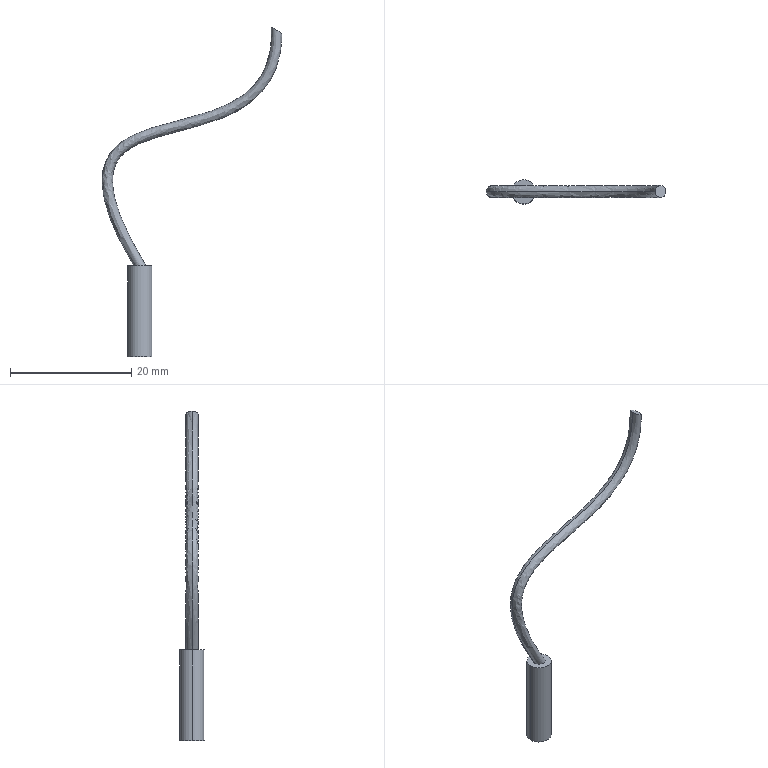Part | STEP file | Rotor detection photoelectric sensor | 1 solid | 7 faces | box 29.674 x 4 x 54.352 mm | volume 340.68 mm3 | plane 3 | spline 2 | cylinder 2 | commonest cylinder face diameters 4 x2
STEP:
#1=CARTESIAN_POINT('',(0.,0.,0.));
#2=DIRECTION('',(0.,0.,1.));
#3=DIRECTION('',(1.,0.,0.));
#4=AXIS2_PLACEMENT_3D('',#1,#2,#3);
#5=CARTESIAN_POINT('',(1.,0.,15.));
#6=VERTEX_POINT('',#5);
#7=CARTESIAN_POINT('',(-1.,0.,15.));
#8=VERTEX_POINT('',#7);
#9=CARTESIAN_POINT('',(1.,0.,15.));
#10=CARTESIAN_POINT('',(1.,2.,15.));
#11=CARTESIAN_POINT('',(-1.,2.,15.));
#12=CARTESIAN_POINT('',(-1.,0.,15.));
#13=(BOUNDED_CURVE()B_SPLINE_CURVE(3,(#9,#10,#11,#12),.UNSPECIFIED.,.F.,.F.)B_SPLINE_CURVE_WITH_KNOTS((4,4),(0.003113,0.006226),.PIECEWISE_BEZIER_KNOTS.)CURVE()GEOMETRIC_REPRESENTATION_ITEM()RATIONAL_B_SPLINE_CURVE((1.,0.3333,0.3333,1.))REPRESENTATION_ITEM(''));
#14=CARTESIAN_POINT('',(1.,0.,15.));
#15=CARTESIAN_POINT('',(0.06152,0.,16.548));
#16=CARTESIAN_POINT('',(-1.541,0.,19.409));
#17=CARTESIAN_POINT('',(-3.194,0.,23.021));
#18=CARTESIAN_POINT('',(-4.04,0.,25.6));
#19=CARTESIAN_POINT('',(-4.414,0.,27.44));
#20=CARTESIAN_POINT('',(-4.535,0.,28.749));
#21=CARTESIAN_POINT('',(-4.495,0.,29.892));
#22=CARTESIAN_POINT('',(-4.265,0.,31.131));
#23=CARTESIAN_POINT('',(-3.713,0.,32.389));
#24=CARTESIAN_POINT('',(-2.639,0.,33.627));
#25=CARTESIAN_POINT('',(-1.142,0.,34.662));
#26=CARTESIAN_POINT('',(2.557,0.,36.372));
#27=CARTESIAN_POINT('',(8.403,0.,37.548));
#28=CARTESIAN_POINT('',(14.934,0.,39.731));
#29=CARTESIAN_POINT('',(18.432,0.,41.83));
#30=CARTESIAN_POINT('',(20.585,0.,44.09));
#31=CARTESIAN_POINT('',(21.786,0.,45.892));
#32=CARTESIAN_POINT('',(22.702,0.,48.014));
#33=CARTESIAN_POINT('',(23.29,0.,50.472));
#34=CARTESIAN_POINT('',(23.436,0.,52.345));
#35=CARTESIAN_POINT('',(23.448,0.,53.346));
#36=CARTESIAN_POINT('',(1.,2.,15.));
#37=CARTESIAN_POINT('',(0.06152,2.,16.548));
#38=CARTESIAN_POINT('',(-1.541,2.,19.409));
#39=CARTESIAN_POINT('',(-3.194,2.,23.021));
#40=CARTESIAN_POINT('',(-4.04,2.,25.6));
#41=CARTESIAN_POINT('',(-4.414,2.,27.44));
#42=CARTESIAN_POINT('',(-4.535,2.,28.749));
#43=CARTESIAN_POINT('',(-4.495,2.,29.892));
#44=CARTESIAN_POINT('',(-4.265,2.,31.131));
#45=CARTESIAN_POINT('',(-3.713,2.,32.389));
#46=CARTESIAN_POINT('',(-2.639,2.,33.627));
#47=CARTESIAN_POINT('',(-1.142,2.,34.662));
#48=CARTESIAN_POINT('',(2.557,2.,36.372));
#49=CARTESIAN_POINT('',(8.403,2.,37.548));
#50=CARTESIAN_POINT('',(14.934,2.,39.731));
#51=CARTESIAN_POINT('',(18.432,2.,41.83));
#52=CARTESIAN_POINT('',(20.585,2.,44.09));
#53=CARTESIAN_POINT('',(21.786,2.,45.892));
#54=CARTESIAN_POINT('',(22.702,2.,48.014));
#55=CARTESIAN_POINT('',(23.29,2.,50.472));
#56=CARTESIAN_POINT('',(23.436,2.,52.345));
#57=CARTESIAN_POINT('',(23.448,2.,53.346));
#58=CARTESIAN_POINT('',(-1.,2.,15.));
#59=CARTESIAN_POINT('',(-1.938,2.,16.594));
#60=CARTESIAN_POINT('',(-3.539,2.,19.546));
#61=CARTESIAN_POINT('',(-5.17,2.,23.359));
#62=CARTESIAN_POINT('',(-5.962,2.,26.177));
#63=CARTESIAN_POINT('',(-6.238,2.,28.273));
#64=CARTESIAN_POINT('',(-6.233,2.,29.819));
#65=CARTESIAN_POINT('',(-6.006,2.,31.216));
#66=CARTESIAN_POINT('',(-5.465,2.,32.757));
#67=CARTESIAN_POINT('',(-4.44,2.,34.283));
#68=CARTESIAN_POINT('',(-2.854,2.,35.631));
#69=CARTESIAN_POINT('',(-0.9914,2.,36.664));
#70=CARTESIAN_POINT('',(3.163,2.,38.3));
#71=CARTESIAN_POINT('',(9.026,2.,39.45));
#72=CARTESIAN_POINT('',(15.16,2.,41.737));
#73=CARTESIAN_POINT('',(18.134,2.,43.837));
#74=CARTESIAN_POINT('',(19.801,2.,45.942));
#75=CARTESIAN_POINT('',(20.686,2.,47.575));
#76=CARTESIAN_POINT('',(21.327,2.,49.479));
#77=CARTESIAN_POINT('',(21.701,2.,51.7));
#78=CARTESIAN_POINT('',(21.754,2.,53.424));
#79=CARTESIAN_POINT('',(21.719,2.,54.352));
#80=CARTESIAN_POINT('',(-1.,0.,15.));
#81=CARTESIAN_POINT('',(-1.938,0.,16.594));
#82=CARTESIAN_POINT('',(-3.539,0.,19.546));
#83=CARTESIAN_POINT('',(-5.17,0.,23.359));
#84=CARTESIAN_POINT('',(-5.962,0.,26.177));
#85=CARTESIAN_POINT('',(-6.238,0.,28.273));
#86=CARTESIAN_POINT('',(-6.233,0.,29.819));
#87=CARTESIAN_POINT('',(-6.006,0.,31.216));
#88=CARTESIAN_POINT('',(-5.465,0.,32.757));
#89=CARTESIAN_POINT('',(-4.44,0.,34.283));
#90=CARTESIAN_POINT('',(-2.854,0.,35.631));
#91=CARTESIAN_POINT('',(-0.9914,0.,36.664));
#92=CARTESIAN_POINT('',(3.163,0.,38.3));
#93=CARTESIAN_POINT('',(9.026,0.,39.45));
#94=CARTESIAN_POINT('',(15.16,0.,41.737));
#95=CARTESIAN_POINT('',(18.134,0.,43.837));
#96=CARTESIAN_POINT('',(19.801,0.,45.942));
#97=CARTESIAN_POINT('',(20.686,0.,47.575));
#98=CARTESIAN_POINT('',(21.327,0.,49.479));
#99=CARTESIAN_POINT('',(21.701,0.,51.7));
#100=CARTESIAN_POINT('',(21.754,0.,53.424));
#101=CARTESIAN_POINT('',(21.719,0.,54.352));
#102=CARTESIAN_POINT('',(-1.,-2.,15.));
#103=CARTESIAN_POINT('',(-1.938,-2.,16.594));
#104=CARTESIAN_POINT('',(-3.539,-2.,19.546));
#105=CARTESIAN_POINT('',(-5.17,-2.,23.359));
#106=CARTESIAN_POINT('',(-5.962,-2.,26.177));
#107=CARTESIAN_POINT('',(-6.238,-2.,28.273));
#108=CARTESIAN_POINT('',(-6.233,-2.,29.819));
#109=CARTESIAN_POINT('',(-6.006,-2.,31.216));
#110=CARTESIAN_POINT('',(-5.465,-2.,32.757));
#111=CARTESIAN_POINT('',(-4.44,-2.,34.283));
#112=CARTESIAN_POINT('',(-2.854,-2.,35.631));
#113=CARTESIAN_POINT('',(-0.9914,-2.,36.664));
#114=CARTESIAN_POINT('',(3.163,-2.,38.3));
#115=CARTESIAN_POINT('',(9.026,-2.,39.45));
#116=CARTESIAN_POINT('',(15.16,-2.,41.737));
#117=CARTESIAN_POINT('',(18.134,-2.,43.837));
#118=CARTESIAN_POINT('',(19.801,-2.,45.942));
#119=CARTESIAN_POINT('',(20.686,-2.,47.575));
#120=CARTESIAN_POINT('',(21.327,-2.,49.479));
#121=CARTESIAN_POINT('',(21.701,-2.,51.7));
#122=CARTESIAN_POINT('',(21.754,-2.,53.424));
#123=CARTESIAN_POINT('',(21.719,-2.,54.352));
#124=CARTESIAN_POINT('',(1.,-2.,15.));
#125=CARTESIAN_POINT('',(0.06152,-2.,16.548));
#126=CARTESIAN_POINT('',(-1.541,-2.,19.409));
#127=CARTESIAN_POINT('',(-3.194,-2.,23.021));
#128=CARTESIAN_POINT('',(-4.04,-2.,25.6));
#129=CARTESIAN_POINT('',(-4.414,-2.,27.44));
#130=CARTESIAN_POINT('',(-4.535,-2.,28.749));
#131=CARTESIAN_POINT('',(-4.495,-2.,29.892));
#132=CARTESIAN_POINT('',(-4.265,-2.,31.131));
#133=CARTESIAN_POINT('',(-3.713,-2.,32.389));
#134=CARTESIAN_POINT('',(-2.639,-2.,33.627));
#135=CARTESIAN_POINT('',(-1.142,-2.,34.662));
#136=CARTESIAN_POINT('',(2.557,-2.,36.372));
#137=CARTESIAN_POINT('',(8.403,-2.,37.548));
#138=CARTESIAN_POINT('',(14.934,-2.,39.731));
#139=CARTESIAN_POINT('',(18.432,-2.,41.83));
#140=CARTESIAN_POINT('',(20.585,-2.,44.09));
#141=CARTESIAN_POINT('',(21.786,-2.,45.892));
#142=CARTESIAN_POINT('',(22.702,-2.,48.014));
#143=CARTESIAN_POINT('',(23.29,-2.,50.472));
#144=CARTESIAN_POINT('',(23.436,-2.,52.345));
#145=CARTESIAN_POINT('',(23.448,-2.,53.346));
#146=CARTESIAN_POINT('',(1.,0.,15.));
#147=CARTESIAN_POINT('',(0.06152,0.,16.548));
#148=CARTESIAN_POINT('',(-1.541,0.,19.409));
#149=CARTESIAN_POINT('',(-3.194,0.,23.021));
#150=CARTESIAN_POINT('',(-4.04,0.,25.6));
#151=CARTESIAN_POINT('',(-4.414,0.,27.44));
#152=CARTESIAN_POINT('',(-4.535,0.,28.749));
#153=CARTESIAN_POINT('',(-4.495,0.,29.892));
#154=CARTESIAN_POINT('',(-4.265,0.,31.131));
#155=CARTESIAN_POINT('',(-3.713,0.,32.389));
#156=CARTESIAN_POINT('',(-2.639,0.,33.627));
#157=CARTESIAN_POINT('',(-1.142,0.,34.662));
#158=CARTESIAN_POINT('',(2.557,0.,36.372));
#159=CARTESIAN_POINT('',(8.403,0.,37.548));
#160=CARTESIAN_POINT('',(14.934,0.,39.731));
#161=CARTESIAN_POINT('',(18.432,0.,41.83));
#162=CARTESIAN_POINT('',(20.585,0.,44.09));
#163=CARTESIAN_POINT('',(21.786,0.,45.892));
#164=CARTESIAN_POINT('',(22.702,0.,48.014));
#165=CARTESIAN_POINT('',(23.29,0.,50.472));
#166=CARTESIAN_POINT('',(23.436,0.,52.345));
#167=CARTESIAN_POINT('',(23.448,0.,53.346));
#168=(BOUNDED_SURFACE()B_SPLINE_SURFACE(3,3,((#14,#15,#16,#17,#18,#19,#20,#21,#22,#23,#24,#25,#26,#27,#28,#29,#30,#31,#32,#33,#34,#35),(#36,#37,#38,#39,#40,#41,#42,#43,#44,#45,#46,#47,#48,#49,#50,#51,#52,#53,#54,#55,#56,#57),(#58,#59,#60,#61,#62,#63,#64,#65,#66,#67,#68,#69,#70,#71,#72,#73,#74,#75,#76,#77,#78,#79),(#80,#81,#82,#83,#84,#85,#86,#87,#88,#89,#90,#91,#92,#93,#94,#95,#96,#97,#98,#99,#100,#101),(#102,#103,#104,#105,#106,#107,#108,#109,#110,#111,#112,#113,#114,#115,#116,#117,#118,#119,#120,#121,#122,#123),(#124,#125,#126,#127,#128,#129,#130,#131,#132,#133,#134,#135,#136,#137,#138,#139,#140,#141,#142,#143,#144,#145),(#146,#147,#148,#149,#150,#151,#152,#153,#154,#155,#156,#157,#158,#159,#160,#161,#162,#163,#164,#165,#166,#167)),.UNSPECIFIED.,.T.,.F.,.F.)B_SPLINE_SURFACE_WITH_KNOTS((1,3,3,3,1),(4,1,1,1,1,1,1,1,1,1,1,1,1,1,1,1,1,1,1,4),(-0.5,0.,0.5,1.,1.5),(0.,0.04667,0.09333,0.14,0.1675,0.195,0.2225,0.25,0.2969,0.3438,0.3906,0.4375,0.625,0.7188,0.8125,0.85,0.8875,0.925,0.9625,1.),.UNSPECIFIED.)GEOMETRIC_REPRESENTATION_ITEM()RATIONAL_B_SPLINE_SURFACE(((1.,1.,1.,1.,1.,1.,1.,1.,1.,1.,1.,1.,1.,1.,1.,1.,1.,1.,1.,1.,1.,1.),(0.3333,0.3333,0.3333,0.3333,0.3333,0.3333,0.3333,0.3333,0.3333,0.3333,0.3333,0.3333,0.3333,0.3333,0.3333,0.3333,0.3333,0.3333,0.3333,0.3333,0.3333,0.3333),(0.3333,0.3333,0.3333,0.3333,0.3333,0.3333,0.3333,0.3333,0.3333,0.3333,0.3333,0.3333,0.3333,0.3333,0.3333,0.3333,0.3333,0.3333,0.3333,0.3333,0.3333,0.3333),(1.,1.,1.,1.,1.,1.,1.,1.,1.,1.,1.,1.,1.,1.,1.,1.,1.,1.,1.,1.,1.,1.),(0.3333,0.3333,0.3333,0.3333,0.3333,0.3333,0.3333,0.3333,0.3333,0.3333,0.3333,0.3333,0.3333,0.3333,0.3333,0.3333,0.3333,0.3333,0.3333,0.3333,0.3333,0.3333),(0.3333,0.3333,0.3333,0.3333,0.3333,0.3333,0.3333,0.3333,0.3333,0.3333,0.3333,0.3333,0.3333,0.3333,0.3333,0.3333,0.3333,0.3333,0.3333,0.3333,0.3333,0.3333),(1.,1.,1.,1.,1.,1.,1.,1.,1.,1.,1.,1.,1.,1.,1.,1.,1.,1.,1.,1.,1.,1.)))REPRESENTATION_ITEM('')SURFACE());
#169=CARTESIAN_POINT('',(0.,0.));
#170=CARTESIAN_POINT('',(0.5,0.));
#171=B_SPLINE_CURVE_WITH_KNOTS('',1,(#169,#170),.UNSPECIFIED.,.F.,.F.,(2,2),(0.003113,0.006226),.PIECEWISE_BEZIER_KNOTS.);
#172=(GEOMETRIC_REPRESENTATION_CONTEXT(2)PARAMETRIC_REPRESENTATION_CONTEXT()REPRESENTATION_CONTEXT('',''));
#173=DEFINITIONAL_REPRESENTATION('',(#171),#172);
#174=PCURVE('',#168,#173);
#175=CARTESIAN_POINT('',(0.,0.,15.));
#176=DIRECTION('',(0.,0.,1.));
#177=DIRECTION('',(1.,0.,0.));
#178=AXIS2_PLACEMENT_3D('',#175,#176,#177);
#179=PLANE('',#178);
#180=CARTESIAN_POINT('',(1.,0.));
#181=CARTESIAN_POINT('',(1.,2.));
#182=CARTESIAN_POINT('',(-1.,2.));
#183=CARTESIAN_POINT('',(-1.,0.));
#184=(BOUNDED_CURVE()B_SPLINE_CURVE(3,(#180,#181,#182,#183),.UNSPECIFIED.,.F.,.F.)B_SPLINE_CURVE_WITH_KNOTS((4,4),(0.003113,0.006226),.PIECEWISE_BEZIER_KNOTS.)CURVE()GEOMETRIC_REPRESENTATION_ITEM()RATIONAL_B_SPLINE_CURVE((1.,0.3333,0.3333,1.))REPRESENTATION_ITEM(''));
#185=(GEOMETRIC_REPRESENTATION_CONTEXT(2)PARAMETRIC_REPRESENTATION_CONTEXT()REPRESENTATION_CONTEXT('',''));
#186=DEFINITIONAL_REPRESENTATION('',(#184),#185);
#187=PCURVE('',#179,#186);
#188=SURFACE_CURVE('',#13,(#174,#187),.PCURVE_S1.);
#189=EDGE_CURVE('',#6,#8,#188,.T.);
#190=ORIENTED_EDGE('',*,*,#189,.T.);
#191=CARTESIAN_POINT('',(21.719,0.,54.352));
#192=VERTEX_POINT('',#191);
#193=CARTESIAN_POINT('',(-1.,0.,15.));
#194=CARTESIAN_POINT('',(-1.938,0.,16.594));
#195=CARTESIAN_POINT('',(-3.539,0.,19.546));
#196=CARTESIAN_POINT('',(-5.17,0.,23.359));
#197=CARTESIAN_POINT('',(-5.962,0.,26.177));
#198=CARTESIAN_POINT('',(-6.238,0.,28.273));
#199=CARTESIAN_POINT('',(-6.233,0.,29.819));
#200=CARTESIAN_POINT('',(-6.006,0.,31.216));
#201=CARTESIAN_POINT('',(-5.465,0.,32.757));
#202=CARTESIAN_POINT('',(-4.44,0.,34.283));
#203=CARTESIAN_POINT('',(-2.854,0.,35.631));
#204=CARTESIAN_POINT('',(-0.9914,0.,36.664));
#205=CARTESIAN_POINT('',(3.163,0.,38.3));
#206=CARTESIAN_POINT('',(9.026,0.,39.45));
#207=CARTESIAN_POINT('',(15.16,0.,41.737));
#208=CARTESIAN_POINT('',(18.134,0.,43.837));
#209=CARTESIAN_POINT('',(19.801,0.,45.942));
#210=CARTESIAN_POINT('',(20.686,0.,47.575));
#211=CARTESIAN_POINT('',(21.327,0.,49.479));
#212=CARTESIAN_POINT('',(21.701,0.,51.7));
#213=CARTESIAN_POINT('',(21.754,0.,53.424));
#214=CARTESIAN_POINT('',(21.719,0.,54.352));
#215=B_SPLINE_CURVE_WITH_KNOTS('',3,(#193,#194,#195,#196,#197,#198,#199,#200,#201,#202,#203,#204,#205,#206,#207,#208,#209,#210,#211,#212,#213,#214),.UNSPECIFIED.,.F.,.F.,(4,1,1,1,1,1,1,1,1,1,1,1,1,1,1,1,1,1,1,4),(0.,0.04667,0.09333,0.14,0.1675,0.195,0.2225,0.25,0.2969,0.3438,0.3906,0.4375,0.625,0.7188,0.8125,0.85,0.8875,0.925,0.9625,1.),.UNSPECIFIED.);
#216=CARTESIAN_POINT('',(0.5,0.));
#217=DIRECTION('',(0.,1.));
#218=VECTOR('',#217,1.);
#219=LINE('',#216,#218);
#220=(GEOMETRIC_REPRESENTATION_CONTEXT(2)PARAMETRIC_REPRESENTATION_CONTEXT()REPRESENTATION_CONTEXT('',''));
#221=DEFINITIONAL_REPRESENTATION('',(#219),#220);
#222=PCURVE('',#168,#221);
#223=CARTESIAN_POINT('',(1.,0.,15.));
#224=CARTESIAN_POINT('',(0.06152,0.,16.548));
#225=CARTESIAN_POINT('',(-1.541,0.,19.409));
#226=CARTESIAN_POINT('',(-3.194,0.,23.021));
#227=CARTESIAN_POINT('',(-4.04,0.,25.6));
#228=CARTESIAN_POINT('',(-4.414,0.,27.44));
#229=CARTESIAN_POINT('',(-4.535,0.,28.749));
#230=CARTESIAN_POINT('',(-4.495,0.,29.892));
#231=CARTESIAN_POINT('',(-4.265,0.,31.131));
#232=CARTESIAN_POINT('',(-3.713,0.,32.389));
#233=CARTESIAN_POINT('',(-2.639,0.,33.627));
#234=CARTESIAN_POINT('',(-1.142,0.,34.662));
#235=CARTESIAN_POINT('',(2.557,0.,36.372));
#236=CARTESIAN_POINT('',(8.403,0.,37.548));
#237=CARTESIAN_POINT('',(14.934,0.,39.731));
#238=CARTESIAN_POINT('',(18.432,0.,41.83));
#239=CARTESIAN_POINT('',(20.585,0.,44.09));
#240=CARTESIAN_POINT('',(21.786,0.,45.892));
#241=CARTESIAN_POINT('',(22.702,0.,48.014));
#242=CARTESIAN_POINT('',(23.29,0.,50.472));
#243=CARTESIAN_POINT('',(23.436,0.,52.345));
#244=CARTESIAN_POINT('',(23.448,0.,53.346));
#245=CARTESIAN_POINT('',(1.,2.,15.));
#246=CARTESIAN_POINT('',(0.06152,2.,16.548));
#247=CARTESIAN_POINT('',(-1.541,2.,19.409));
#248=CARTESIAN_POINT('',(-3.194,2.,23.021));
#249=CARTESIAN_POINT('',(-4.04,2.,25.6));
#250=CARTESIAN_POINT('',(-4.414,2.,27.44));
#251=CARTESIAN_POINT('',(-4.535,2.,28.749));
#252=CARTESIAN_POINT('',(-4.495,2.,29.892));
#253=CARTESIAN_POINT('',(-4.265,2.,31.131));
#254=CARTESIAN_POINT('',(-3.713,2.,32.389));
#255=CARTESIAN_POINT('',(-2.639,2.,33.627));
#256=CARTESIAN_POINT('',(-1.142,2.,34.662));
#257=CARTESIAN_POINT('',(2.557,2.,36.372));
#258=CARTESIAN_POINT('',(8.403,2.,37.548));
#259=CARTESIAN_POINT('',(14.934,2.,39.731));
#260=CARTESIAN_POINT('',(18.432,2.,41.83));
#261=CARTESIAN_POINT('',(20.585,2.,44.09));
#262=CARTESIAN_POINT('',(21.786,2.,45.892));
#263=CARTESIAN_POINT('',(22.702,2.,48.014));
#264=CARTESIAN_POINT('',(23.29,2.,50.472));
#265=CARTESIAN_POINT('',(23.436,2.,52.345));
#266=CARTESIAN_POINT('',(23.448,2.,53.346));
#267=CARTESIAN_POINT('',(-1.,2.,15.));
#268=CARTESIAN_POINT('',(-1.938,2.,16.594));
#269=CARTESIAN_POINT('',(-3.539,2.,19.546));
#270=CARTESIAN_POINT('',(-5.17,2.,23.359));
#271=CARTESIAN_POINT('',(-5.962,2.,26.177));
#272=CARTESIAN_POINT('',(-6.238,2.,28.273));
#273=CARTESIAN_POINT('',(-6.233,2.,29.819));
#274=CARTESIAN_POINT('',(-6.006,2.,31.216));
#275=CARTESIAN_POINT('',(-5.465,2.,32.757));
#276=CARTESIAN_POINT('',(-4.44,2.,34.283));
#277=CARTESIAN_POINT('',(-2.854,2.,35.631));
#278=CARTESIAN_POINT('',(-0.9914,2.,36.664));
#279=CARTESIAN_POINT('',(3.163,2.,38.3));
#280=CARTESIAN_POINT('',(9.026,2.,39.45));
#281=CARTESIAN_POINT('',(15.16,2.,41.737));
#282=CARTESIAN_POINT('',(18.134,2.,43.837));
#283=CARTESIAN_POINT('',(19.801,2.,45.942));
#284=CARTESIAN_POINT('',(20.686,2.,47.575));
#285=CARTESIAN_POINT('',(21.327,2.,49.479));
#286=CARTESIAN_POINT('',(21.701,2.,51.7));
#287=CARTESIAN_POINT('',(21.754,2.,53.424));
#288=CARTESIAN_POINT('',(21.719,2.,54.352));
#289=CARTESIAN_POINT('',(-1.,0.,15.));
#290=CARTESIAN_POINT('',(-1.938,0.,16.594));
#291=CARTESIAN_POINT('',(-3.539,0.,19.546));
#292=CARTESIAN_POINT('',(-5.17,0.,23.359));
#293=CARTESIAN_POINT('',(-5.962,0.,26.177));
#294=CARTESIAN_POINT('',(-6.238,0.,28.273));
#295=CARTESIAN_POINT('',(-6.233,0.,29.819));
#296=CARTESIAN_POINT('',(-6.006,0.,31.216));
#297=CARTESIAN_POINT('',(-5.465,0.,32.757));
#298=CARTESIAN_POINT('',(-4.44,0.,34.283));
#299=CARTESIAN_POINT('',(-2.854,0.,35.631));
#300=CARTESIAN_POINT('',(-0.9914,0.,36.664));
#301=CARTESIAN_POINT('',(3.163,0.,38.3));
#302=CARTESIAN_POINT('',(9.026,0.,39.45));
#303=CARTESIAN_POINT('',(15.16,0.,41.737));
#304=CARTESIAN_POINT('',(18.134,0.,43.837));
#305=CARTESIAN_POINT('',(19.801,0.,45.942));
#306=CARTESIAN_POINT('',(20.686,0.,47.575));
#307=CARTESIAN_POINT('',(21.327,0.,49.479));
#308=CARTESIAN_POINT('',(21.701,0.,51.7));
#309=CARTESIAN_POINT('',(21.754,0.,53.424));
#310=CARTESIAN_POINT('',(21.719,0.,54.352));
#311=CARTESIAN_POINT('',(-1.,-2.,15.));
#312=CARTESIAN_POINT('',(-1.938,-2.,16.594));
#313=CARTESIAN_POINT('',(-3.539,-2.,19.546));
#314=CARTESIAN_POINT('',(-5.17,-2.,23.359));
#315=CARTESIAN_POINT('',(-5.962,-2.,26.177));
#316=CARTESIAN_POINT('',(-6.238,-2.,28.273));
#317=CARTESIAN_POINT('',(-6.233,-2.,29.819));
#318=CARTESIAN_POINT('',(-6.006,-2.,31.216));
#319=CARTESIAN_POINT('',(-5.465,-2.,32.757));
#320=CARTESIAN_POINT('',(-4.44,-2.,34.283));
#321=CARTESIAN_POINT('',(-2.854,-2.,35.631));
#322=CARTESIAN_POINT('',(-0.9914,-2.,36.664));
#323=CARTESIAN_POINT('',(3.163,-2.,38.3));
#324=CARTESIAN_POINT('',(9.026,-2.,39.45));
#325=CARTESIAN_POINT('',(15.16,-2.,41.737));
#326=CARTESIAN_POINT('',(18.134,-2.,43.837));
#327=CARTESIAN_POINT('',(19.801,-2.,45.942));
#328=CARTESIAN_POINT('',(20.686,-2.,47.575));
#329=CARTESIAN_POINT('',(21.327,-2.,49.479));
#330=CARTESIAN_POINT('',(21.701,-2.,51.7));
#331=CARTESIAN_POINT('',(21.754,-2.,53.424));
#332=CARTESIAN_POINT('',(21.719,-2.,54.352));
#333=CARTESIAN_POINT('',(1.,-2.,15.));
#334=CARTESIAN_POINT('',(0.06152,-2.,16.548));
#335=CARTESIAN_POINT('',(-1.541,-2.,19.409));
#336=CARTESIAN_POINT('',(-3.194,-2.,23.021));
#337=CARTESIAN_POINT('',(-4.04,-2.,25.6));
#338=CARTESIAN_POINT('',(-4.414,-2.,27.44));
#339=CARTESIAN_POINT('',(-4.535,-2.,28.749));
#340=CARTESIAN_POINT('',(-4.495,-2.,29.892));
#341=CARTESIAN_POINT('',(-4.265,-2.,31.131));
#342=CARTESIAN_POINT('',(-3.713,-2.,32.389));
#343=CARTESIAN_POINT('',(-2.639,-2.,33.627));
#344=CARTESIAN_POINT('',(-1.142,-2.,34.662));
#345=CARTESIAN_POINT('',(2.557,-2.,36.372));
#346=CARTESIAN_POINT('',(8.403,-2.,37.548));
#347=CARTESIAN_POINT('',(14.934,-2.,39.731));
#348=CARTESIAN_POINT('',(18.432,-2.,41.83));
#349=CARTESIAN_POINT('',(20.585,-2.,44.09));
#350=CARTESIAN_POINT('',(21.786,-2.,45.892));
#351=CARTESIAN_POINT('',(22.702,-2.,48.014));
#352=CARTESIAN_POINT('',(23.29,-2.,50.472));
#353=CARTESIAN_POINT('',(23.436,-2.,52.345));
#354=CARTESIAN_POINT('',(23.448,-2.,53.346));
#355=CARTESIAN_POINT('',(1.,0.,15.));
#356=CARTESIAN_POINT('',(0.06152,0.,16.548));
#357=CARTESIAN_POINT('',(-1.541,0.,19.409));
#358=CARTESIAN_POINT('',(-3.194,0.,23.021));
#359=CARTESIAN_POINT('',(-4.04,0.,25.6));
#360=CARTESIAN_POINT('',(-4.414,0.,27.44));
#361=CARTESIAN_POINT('',(-4.535,0.,28.749));
#362=CARTESIAN_POINT('',(-4.495,0.,29.892));
#363=CARTESIAN_POINT('',(-4.265,0.,31.131));
#364=CARTESIAN_POINT('',(-3.713,0.,32.389));
#365=CARTESIAN_POINT('',(-2.639,0.,33.627));
#366=CARTESIAN_POINT('',(-1.142,0.,34.662));
#367=CARTESIAN_POINT('',(2.557,0.,36.372));
#368=CARTESIAN_POINT('',(8.403,0.,37.548));
#369=CARTESIAN_POINT('',(14.934,0.,39.731));
#370=CARTESIAN_POINT('',(18.432,0.,41.83));
#371=CARTESIAN_POINT('',(20.585,0.,44.09));
#372=CARTESIAN_POINT('',(21.786,0.,45.892));
#373=CARTESIAN_POINT('',(22.702,0.,48.014));
#374=CARTESIAN_POINT('',(23.29,0.,50.472));
#375=CARTESIAN_POINT('',(23.436,0.,52.345));
#376=CARTESIAN_POINT('',(23.448,0.,53.346));
#377=(BOUNDED_SURFACE()B_SPLINE_SURFACE(3,3,((#223,#224,#225,#226,#227,#228,#229,#230,#231,#232,#233,#234,#235,#236,#237,#238,#239,#240,#241,#242,#243,#244),(#245,#246,#247,#248,#249,#250,#251,#252,#253,#254,#255,#256,#257,#258,#259,#260,#261,#262,#263,#264,#265,#266),(#267,#268,#269,#270,#271,#272,#273,#274,#275,#276,#277,#278,#279,#280,#281,#282,#283,#284,#285,#286,#287,#288),(#289,#290,#291,#292,#293,#294,#295,#296,#297,#298,#299,#300,#301,#302,#303,#304,#305,#306,#307,#308,#309,#310),(#311,#312,#313,#314,#315,#316,#317,#318,#319,#320,#321,#322,#323,#324,#325,#326,#327,#328,#329,#330,#331,#332),(#333,#334,#335,#336,#337,#338,#339,#340,#341,#342,#343,#344,#345,#346,#347,#348,#349,#350,#351,#352,#353,#354),(#355,#356,#357,#358,#359,#360,#361,#362,#363,#364,#365,#366,#367,#368,#369,#370,#371,#372,#373,#374,#375,#376)),.UNSPECIFIED.,.T.,.F.,.F.)B_SPLINE_SURFACE_WITH_KNOTS((1,3,3,3,1),(4,1,1,1,1,1,1,1,1,1,1,1,1,1,1,1,1,1,1,4),(-0.5,0.,0.5,1.,1.5),(0.,0.04667,0.09333,0.14,0.1675,0.195,0.2225,0.25,0.2969,0.3438,0.3906,0.4375,0.625,0.7188,0.8125,0.85,0.8875,0.925,0.9625,1.),.UNSPECIFIED.)GEOMETRIC_REPRESENTATION_ITEM()RATIONAL_B_SPLINE_SURFACE(((1.,1.,1.,1.,1.,1.,1.,1.,1.,1.,1.,1.,1.,1.,1.,1.,1.,1.,1.,1.,1.,1.),(0.3333,0.3333,0.3333,0.3333,0.3333,0.3333,0.3333,0.3333,0.3333,0.3333,0.3333,0.3333,0.3333,0.3333,0.3333,0.3333,0.3333,0.3333,0.3333,0.3333,0.3333,0.3333),(0.3333,0.3333,0.3333,0.3333,0.3333,0.3333,0.3333,0.3333,0.3333,0.3333,0.3333,0.3333,0.3333,0.3333,0.3333,0.3333,0.3333,0.3333,0.3333,0.3333,0.3333,0.3333),(1.,1.,1.,1.,1.,1.,1.,1.,1.,1.,1.,1.,1.,1.,1.,1.,1.,1.,1.,1.,1.,1.),(0.3333,0.3333,0.3333,0.3333,0.3333,0.3333,0.3333,0.3333,0.3333,0.3333,0.3333,0.3333,0.3333,0.3333,0.3333,0.3333,0.3333,0.3333,0.3333,0.3333,0.3333,0.3333),(0.3333,0.3333,0.3333,0.3333,0.3333,0.3333,0.3333,0.3333,0.3333,0.3333,0.3333,0.3333,0.3333,0.3333,0.3333,0.3333,0.3333,0.3333,0.3333,0.3333,0.3333,0.3333),(1.,1.,1.,1.,1.,1.,1.,1.,1.,1.,1.,1.,1.,1.,1.,1.,1.,1.,1.,1.,1.,1.)))REPRESENTATION_ITEM('')SURFACE());
#378=CARTESIAN_POINT('',(0.5,0.));
#379=DIRECTION('',(0.,1.));
#380=VECTOR('',#379,1.);
#381=LINE('',#378,#380);
#382=(GEOMETRIC_REPRESENTATION_CONTEXT(2)PARAMETRIC_REPRESENTATION_CONTEXT()REPRESENTATION_CONTEXT('',''));
#383=DEFINITIONAL_REPRESENTATION('',(#381),#382);
#384=PCURVE('',#377,#383);
#385=SURFACE_CURVE('',#215,(#222,#384),.PCURVE_S1.);
#386=EDGE_CURVE('',#8,#192,#385,.T.);
#387=ORIENTED_EDGE('',*,*,#386,.T.);
#388=CARTESIAN_POINT('',(23.448,0.,53.346));
#389=VERTEX_POINT('',#388);
#390=CARTESIAN_POINT('',(21.719,0.,54.352));
#391=CARTESIAN_POINT('',(21.719,2.,54.352));
#392=CARTESIAN_POINT('',(23.448,2.,53.346));
#393=CARTESIAN_POINT('',(23.448,0.,53.346));
#394=(BOUNDED_CURVE()B_SPLINE_CURVE(3,(#390,#391,#392,#393),.UNSPECIFIED.,.F.,.F.)B_SPLINE_CURVE_WITH_KNOTS((4,4),(0.003113,0.006226),.PIECEWISE_BEZIER_KNOTS.)CURVE()GEOMETRIC_REPRESENTATION_ITEM()RATIONAL_B_SPLINE_CURVE((1.,0.3333,0.3333,1.))REPRESENTATION_ITEM(''));
#395=CARTESIAN_POINT('',(0.5,1.));
#396=CARTESIAN_POINT('',(0.,1.));
#397=B_SPLINE_CURVE_WITH_KNOTS('',1,(#395,#396),.UNSPECIFIED.,.F.,.F.,(2,2),(0.003113,0.006226),.PIECEWISE_BEZIER_KNOTS.);
#398=(GEOMETRIC_REPRESENTATION_CONTEXT(2)PARAMETRIC_REPRESENTATION_CONTEXT()REPRESENTATION_CONTEXT('',''));
#399=DEFINITIONAL_REPRESENTATION('',(#397),#398);
#400=PCURVE('',#168,#399);
#401=CARTESIAN_POINT('',(21.719,0.,54.352));
#402=DIRECTION('',(-0.5027,0.,-0.8644));
#403=DIRECTION('',(-0.8644,0.,0.5027));
#404=AXIS2_PLACEMENT_3D('',#401,#402,#403);
#405=PLANE('',#404);
#406=CARTESIAN_POINT('',(0.,0.));
#407=CARTESIAN_POINT('',(0.,2.));
#408=CARTESIAN_POINT('',(-2.,2.));
#409=CARTESIAN_POINT('',(-2.,0.));
#410=(BOUNDED_CURVE()B_SPLINE_CURVE(3,(#406,#407,#408,#409),.UNSPECIFIED.,.F.,.F.)B_SPLINE_CURVE_WITH_KNOTS((4,4),(0.003113,0.006226),.PIECEWISE_BEZIER_KNOTS.)CURVE()GEOMETRIC_REPRESENTATION_ITEM()RATIONAL_B_SPLINE_CURVE((1.,0.3333,0.3333,1.))REPRESENTATION_ITEM(''));
#411=(GEOMETRIC_REPRESENTATION_CONTEXT(2)PARAMETRIC_REPRESENTATION_CONTEXT()REPRESENTATION_CONTEXT('',''));
#412=DEFINITIONAL_REPRESENTATION('',(#410),#411);
#413=PCURVE('',#405,#412);
#414=SURFACE_CURVE('',#394,(#400,#413),.PCURVE_S1.);
#415=EDGE_CURVE('',#192,#389,#414,.T.);
#416=ORIENTED_EDGE('',*,*,#415,.T.);
#417=CARTESIAN_POINT('',(1.,0.,15.));
#418=CARTESIAN_POINT('',(0.06152,0.,16.548));
#419=CARTESIAN_POINT('',(-1.541,0.,19.409));
#420=CARTESIAN_POINT('',(-3.194,0.,23.021));
#421=CARTESIAN_POINT('',(-4.04,0.,25.6));
#422=CARTESIAN_POINT('',(-4.414,0.,27.44));
#423=CARTESIAN_POINT('',(-4.535,0.,28.749));
#424=CARTESIAN_POINT('',(-4.495,0.,29.892));
#425=CARTESIAN_POINT('',(-4.265,0.,31.131));
#426=CARTESIAN_POINT('',(-3.713,0.,32.389));
#427=CARTESIAN_POINT('',(-2.639,0.,33.627));
#428=CARTESIAN_POINT('',(-1.142,0.,34.662));
#429=CARTESIAN_POINT('',(2.557,0.,36.372));
#430=CARTESIAN_POINT('',(8.403,0.,37.548));
#431=CARTESIAN_POINT('',(14.934,0.,39.731));
#432=CARTESIAN_POINT('',(18.432,0.,41.83));
#433=CARTESIAN_POINT('',(20.585,0.,44.09));
#434=CARTESIAN_POINT('',(21.786,0.,45.892));
#435=CARTESIAN_POINT('',(22.702,0.,48.014));
#436=CARTESIAN_POINT('',(23.29,0.,50.472));
#437=CARTESIAN_POINT('',(23.436,0.,52.345));
#438=CARTESIAN_POINT('',(23.448,0.,53.346));
#439=B_SPLINE_CURVE_WITH_KNOTS('',3,(#417,#418,#419,#420,#421,#422,#423,#424,#425,#426,#427,#428,#429,#430,#431,#432,#433,#434,#435,#436,#437,#438),.UNSPECIFIED.,.F.,.F.,(4,1,1,1,1,1,1,1,1,1,1,1,1,1,1,1,1,1,1,4),(0.,0.04667,0.09333,0.14,0.1675,0.195,0.2225,0.25,0.2969,0.3438,0.3906,0.4375,0.625,0.7188,0.8125,0.85,0.8875,0.925,0.9625,1.),.UNSPECIFIED.);
#440=CARTESIAN_POINT('',(0.,0.));
#441=DIRECTION('',(0.,1.));
#442=VECTOR('',#441,1.);
#443=LINE('',#440,#442);
#444=(GEOMETRIC_REPRESENTATION_CONTEXT(2)PARAMETRIC_REPRESENTATION_CONTEXT()REPRESENTATION_CONTEXT('',''));
#445=DEFINITIONAL_REPRESENTATION('',(#443),#444);
#446=PCURVE('',#168,#445);
#447=CARTESIAN_POINT('',(1.,0.));
#448=DIRECTION('',(0.,1.));
#449=VECTOR('',#448,1.);
#450=LINE('',#447,#449);
#451=(GEOMETRIC_REPRESENTATION_CONTEXT(2)PARAMETRIC_REPRESENTATION_CONTEXT()REPRESENTATION_CONTEXT('',''));
#452=DEFINITIONAL_REPRESENTATION('',(#450),#451);
#453=PCURVE('',#377,#452);
#454=SURFACE_CURVE('',#439,(#446,#453),.PCURVE_S1.);
#455=EDGE_CURVE('',#6,#389,#454,.T.);
#456=ORIENTED_EDGE('',*,*,#455,.F.);
#457=EDGE_LOOP('',(#190,#387,#416,#456));
#458=FACE_BOUND('',#457,.T.);
#459=ADVANCED_FACE('',(#458),#168,.T.);
#460=CARTESIAN_POINT('',(2.,0.,15.));
#461=VERTEX_POINT('',#460);
#462=CARTESIAN_POINT('',(-2.,0.,15.));
#463=VERTEX_POINT('',#462);
#464=CARTESIAN_POINT('',(0.,0.,15.));
#465=DIRECTION('',(0.,0.,1.));
#466=DIRECTION('',(-1.,0.,0.));
#467=AXIS2_PLACEMENT_3D('',#464,#465,#466);
#468=CIRCLE('',#467,2.);
#469=CARTESIAN_POINT('',(0.,0.,15.));
#470=DIRECTION('',(0.,0.,-1.));
#471=DIRECTION('',(-1.,0.,0.));
#472=AXIS2_PLACEMENT_3D('',#469,#470,#471);
#473=CYLINDRICAL_SURFACE('',#472,2.);
#474=CARTESIAN_POINT('',(6.283,0.));
#475=DIRECTION('',(-1.,0.));
#476=VECTOR('',#475,1.);
#477=LINE('',#474,#476);
#478=(GEOMETRIC_REPRESENTATION_CONTEXT(2)PARAMETRIC_REPRESENTATION_CONTEXT()REPRESENTATION_CONTEXT('',''));
#479=DEFINITIONAL_REPRESENTATION('',(#477),#478);
#480=PCURVE('',#473,#479);
#481=CARTESIAN_POINT('',(0.,0.));
#482=DIRECTION('',(-1.,0.));
#483=AXIS2_PLACEMENT_2D('',#481,#482);
#484=CIRCLE('',#483,2.);
#485=(GEOMETRIC_REPRESENTATION_CONTEXT(2)PARAMETRIC_REPRESENTATION_CONTEXT()REPRESENTATION_CONTEXT('',''));
#486=DEFINITIONAL_REPRESENTATION('',(#484),#485);
#487=PCURVE('',#179,#486);
#488=SURFACE_CURVE('',#468,(#480,#487),.PCURVE_S1.);
#489=EDGE_CURVE('',#461,#463,#488,.T.);
#490=ORIENTED_EDGE('',*,*,#489,.F.);
#491=CARTESIAN_POINT('',(2.,0.,0.));
#492=VERTEX_POINT('',#491);
#493=CARTESIAN_POINT('',(2.,0.,15.));
#494=DIRECTION('',(0.,0.,-1.));
#495=VECTOR('',#494,1.);
#496=LINE('',#493,#495);
#497=CARTESIAN_POINT('',(3.142,0.));
#498=DIRECTION('',(0.,1.));
#499=VECTOR('',#498,1.);
#500=LINE('',#497,#499);
#501=(GEOMETRIC_REPRESENTATION_CONTEXT(2)PARAMETRIC_REPRESENTATION_CONTEXT()REPRESENTATION_CONTEXT('',''));
#502=DEFINITIONAL_REPRESENTATION('',(#500),#501);
#503=PCURVE('',#473,#502);
#504=CARTESIAN_POINT('',(0.,0.,15.));
#505=DIRECTION('',(0.,0.,-1.));
#506=DIRECTION('',(-1.,0.,0.));
#507=AXIS2_PLACEMENT_3D('',#504,#505,#506);
#508=CYLINDRICAL_SURFACE('',#507,2.);
#509=CARTESIAN_POINT('',(3.142,0.));
#510=DIRECTION('',(0.,1.));
#511=VECTOR('',#510,1.);
#512=LINE('',#509,#511);
#513=(GEOMETRIC_REPRESENTATION_CONTEXT(2)PARAMETRIC_REPRESENTATION_CONTEXT()REPRESENTATION_CONTEXT('',''));
#514=DEFINITIONAL_REPRESENTATION('',(#512),#513);
#515=PCURVE('',#508,#514);
#516=SURFACE_CURVE('',#496,(#503,#515),.PCURVE_S1.);
#517=EDGE_CURVE('',#461,#492,#516,.T.);
#518=ORIENTED_EDGE('',*,*,#517,.T.);
#519=CARTESIAN_POINT('',(-2.,0.,0.));
#520=VERTEX_POINT('',#519);
#521=CARTESIAN_POINT('',(0.,0.,0.));
#522=DIRECTION('',(0.,0.,1.));
#523=DIRECTION('',(-1.,0.,0.));
#524=AXIS2_PLACEMENT_3D('',#521,#522,#523);
#525=CIRCLE('',#524,2.);
#526=CARTESIAN_POINT('',(6.283,15.));
#527=DIRECTION('',(-1.,0.));
#528=VECTOR('',#527,1.);
#529=LINE('',#526,#528);
#530=(GEOMETRIC_REPRESENTATION_CONTEXT(2)PARAMETRIC_REPRESENTATION_CONTEXT()REPRESENTATION_CONTEXT('',''));
#531=DEFINITIONAL_REPRESENTATION('',(#529),#530);
#532=PCURVE('',#473,#531);
#533=CARTESIAN_POINT('',(0.,0.,0.));
#534=DIRECTION('',(0.,0.,1.));
#535=DIRECTION('',(1.,0.,0.));
#536=AXIS2_PLACEMENT_3D('',#533,#534,#535);
#537=PLANE('',#536);
#538=CARTESIAN_POINT('',(0.,0.));
#539=DIRECTION('',(-1.,0.));
#540=AXIS2_PLACEMENT_2D('',#538,#539);
#541=CIRCLE('',#540,2.);
#542=(GEOMETRIC_REPRESENTATION_CONTEXT(2)PARAMETRIC_REPRESENTATION_CONTEXT()REPRESENTATION_CONTEXT('',''));
#543=DEFINITIONAL_REPRESENTATION('',(#541),#542);
#544=PCURVE('',#537,#543);
#545=SURFACE_CURVE('',#525,(#532,#544),.PCURVE_S1.);
#546=EDGE_CURVE('',#492,#520,#545,.T.);
#547=ORIENTED_EDGE('',*,*,#546,.T.);
#548=CARTESIAN_POINT('',(-2.,0.,15.));
#549=DIRECTION('',(0.,0.,-1.));
#550=VECTOR('',#549,1.);
#551=LINE('',#548,#550);
#552=CARTESIAN_POINT('',(0.,0.));
#553=DIRECTION('',(0.,1.));
#554=VECTOR('',#553,1.);
#555=LINE('',#552,#554);
#556=(GEOMETRIC_REPRESENTATION_CONTEXT(2)PARAMETRIC_REPRESENTATION_CONTEXT()REPRESENTATION_CONTEXT('',''));
#557=DEFINITIONAL_REPRESENTATION('',(#555),#556);
#558=PCURVE('',#473,#557);
#559=CARTESIAN_POINT('',(6.283,0.));
#560=DIRECTION('',(0.,1.));
#561=VECTOR('',#560,1.);
#562=LINE('',#559,#561);
#563=(GEOMETRIC_REPRESENTATION_CONTEXT(2)PARAMETRIC_REPRESENTATION_CONTEXT()REPRESENTATION_CONTEXT('',''));
#564=DEFINITIONAL_REPRESENTATION('',(#562),#563);
#565=PCURVE('',#508,#564);
#566=SURFACE_CURVE('',#551,(#558,#565),.PCURVE_S1.);
#567=EDGE_CURVE('',#463,#520,#566,.T.);
#568=ORIENTED_EDGE('',*,*,#567,.F.);
#569=EDGE_LOOP('',(#490,#518,#547,#568));
#570=FACE_BOUND('',#569,.T.);
#571=ADVANCED_FACE('',(#570),#473,.T.);
#572=ORIENTED_EDGE('',*,*,#386,.F.);
#573=CARTESIAN_POINT('',(-1.,0.,15.));
#574=CARTESIAN_POINT('',(-1.,-2.,15.));
#575=CARTESIAN_POINT('',(1.,-2.,15.));
#576=CARTESIAN_POINT('',(1.,0.,15.));
#577=(BOUNDED_CURVE()B_SPLINE_CURVE(3,(#573,#574,#575,#576),.UNSPECIFIED.,.F.,.F.)B_SPLINE_CURVE_WITH_KNOTS((4,4),(0.,0.003113),.PIECEWISE_BEZIER_KNOTS.)CURVE()GEOMETRIC_REPRESENTATION_ITEM()RATIONAL_B_SPLINE_CURVE((1.,0.3333,0.3333,1.))REPRESENTATION_ITEM(''));
#578=CARTESIAN_POINT('',(0.5,0.));
#579=CARTESIAN_POINT('',(1.,0.));
#580=B_SPLINE_CURVE_WITH_KNOTS('',1,(#578,#579),.UNSPECIFIED.,.F.,.F.,(2,2),(0.,0.003113),.PIECEWISE_BEZIER_KNOTS.);
#581=(GEOMETRIC_REPRESENTATION_CONTEXT(2)PARAMETRIC_REPRESENTATION_CONTEXT()REPRESENTATION_CONTEXT('',''));
#582=DEFINITIONAL_REPRESENTATION('',(#580),#581);
#583=PCURVE('',#377,#582);
#584=CARTESIAN_POINT('',(-1.,0.));
#585=CARTESIAN_POINT('',(-1.,-2.));
#586=CARTESIAN_POINT('',(1.,-2.));
#587=CARTESIAN_POINT('',(1.,0.));
#588=(BOUNDED_CURVE()B_SPLINE_CURVE(3,(#584,#585,#586,#587),.UNSPECIFIED.,.F.,.F.)B_SPLINE_CURVE_WITH_KNOTS((4,4),(0.,0.003113),.PIECEWISE_BEZIER_KNOTS.)CURVE()GEOMETRIC_REPRESENTATION_ITEM()RATIONAL_B_SPLINE_CURVE((1.,0.3333,0.3333,1.))REPRESENTATION_ITEM(''));
#589=(GEOMETRIC_REPRESENTATION_CONTEXT(2)PARAMETRIC_REPRESENTATION_CONTEXT()REPRESENTATION_CONTEXT('',''));
#590=DEFINITIONAL_REPRESENTATION('',(#588),#589);
#591=PCURVE('',#179,#590);
#592=SURFACE_CURVE('',#577,(#583,#591),.PCURVE_S1.);
#593=EDGE_CURVE('',#8,#6,#592,.T.);
#594=ORIENTED_EDGE('',*,*,#593,.T.);
#595=ORIENTED_EDGE('',*,*,#455,.T.);
#596=CARTESIAN_POINT('',(23.448,0.,53.346));
#597=CARTESIAN_POINT('',(23.448,-2.,53.346));
#598=CARTESIAN_POINT('',(21.719,-2.,54.352));
#599=CARTESIAN_POINT('',(21.719,0.,54.352));
#600=(BOUNDED_CURVE()B_SPLINE_CURVE(3,(#596,#597,#598,#599),.UNSPECIFIED.,.F.,.F.)B_SPLINE_CURVE_WITH_KNOTS((4,4),(0.,0.003113),.PIECEWISE_BEZIER_KNOTS.)CURVE()GEOMETRIC_REPRESENTATION_ITEM()RATIONAL_B_SPLINE_CURVE((1.,0.3333,0.3333,1.))REPRESENTATION_ITEM(''));
#601=CARTESIAN_POINT('',(1.,1.));
#602=CARTESIAN_POINT('',(0.5,1.));
#603=B_SPLINE_CURVE_WITH_KNOTS('',1,(#601,#602),.UNSPECIFIED.,.F.,.F.,(2,2),(0.,0.003113),.PIECEWISE_BEZIER_KNOTS.);
#604=(GEOMETRIC_REPRESENTATION_CONTEXT(2)PARAMETRIC_REPRESENTATION_CONTEXT()REPRESENTATION_CONTEXT('',''));
#605=DEFINITIONAL_REPRESENTATION('',(#603),#604);
#606=PCURVE('',#377,#605);
#607=CARTESIAN_POINT('',(-2.,0.));
#608=CARTESIAN_POINT('',(-2.,-2.));
#609=CARTESIAN_POINT('',(0.,-2.));
#610=CARTESIAN_POINT('',(0.,0.));
#611=(BOUNDED_CURVE()B_SPLINE_CURVE(3,(#607,#608,#609,#610),.UNSPECIFIED.,.F.,.F.)B_SPLINE_CURVE_WITH_KNOTS((4,4),(0.,0.003113),.PIECEWISE_BEZIER_KNOTS.)CURVE()GEOMETRIC_REPRESENTATION_ITEM()RATIONAL_B_SPLINE_CURVE((1.,0.3333,0.3333,1.))REPRESENTATION_ITEM(''));
#612=(GEOMETRIC_REPRESENTATION_CONTEXT(2)PARAMETRIC_REPRESENTATION_CONTEXT()REPRESENTATION_CONTEXT('',''));
#613=DEFINITIONAL_REPRESENTATION('',(#611),#612);
#614=PCURVE('',#405,#613);
#615=SURFACE_CURVE('',#600,(#606,#614),.PCURVE_S1.);
#616=EDGE_CURVE('',#389,#192,#615,.T.);
#617=ORIENTED_EDGE('',*,*,#616,.T.);
#618=EDGE_LOOP('',(#572,#594,#595,#617));
#619=FACE_BOUND('',#618,.T.);
#620=ADVANCED_FACE('',(#619),#377,.T.);
#621=ORIENTED_EDGE('',*,*,#616,.F.);
#622=ORIENTED_EDGE('',*,*,#415,.F.);
#623=EDGE_LOOP('',(#621,#622));
#624=FACE_BOUND('',#623,.T.);
#625=ADVANCED_FACE('',(#624),#405,.F.);
#626=CARTESIAN_POINT('',(0.,0.,15.));
#627=DIRECTION('',(0.,0.,1.));
#628=DIRECTION('',(-1.,0.,0.));
#629=AXIS2_PLACEMENT_3D('',#626,#627,#628);
#630=CIRCLE('',#629,2.);
#631=CARTESIAN_POINT('',(0.,0.));
#632=DIRECTION('',(-1.,0.));
#633=AXIS2_PLACEMENT_2D('',#631,#632);
#634=CIRCLE('',#633,2.);
#635=(GEOMETRIC_REPRESENTATION_CONTEXT(2)PARAMETRIC_REPRESENTATION_CONTEXT()REPRESENTATION_CONTEXT('',''));
#636=DEFINITIONAL_REPRESENTATION('',(#634),#635);
#637=PCURVE('',#179,#636);
#638=CARTESIAN_POINT('',(6.283,0.));
#639=DIRECTION('',(-1.,0.));
#640=VECTOR('',#639,1.);
#641=LINE('',#638,#640);
#642=(GEOMETRIC_REPRESENTATION_CONTEXT(2)PARAMETRIC_REPRESENTATION_CONTEXT()REPRESENTATION_CONTEXT('',''));
#643=DEFINITIONAL_REPRESENTATION('',(#641),#642);
#644=PCURVE('',#508,#643);
#645=SURFACE_CURVE('',#630,(#637,#644),.PCURVE_S1.);
#646=EDGE_CURVE('',#463,#461,#645,.T.);
#647=ORIENTED_EDGE('',*,*,#646,.T.);
#648=ORIENTED_EDGE('',*,*,#489,.T.);
#649=EDGE_LOOP('',(#647,#648));
#650=FACE_BOUND('',#649,.T.);
#651=ORIENTED_EDGE('',*,*,#189,.F.);
#652=ORIENTED_EDGE('',*,*,#593,.F.);
#653=EDGE_LOOP('',(#651,#652));
#654=FACE_BOUND('',#653,.T.);
#655=ADVANCED_FACE('',(#650,#654),#179,.T.);
#656=ORIENTED_EDGE('',*,*,#517,.F.);
#657=ORIENTED_EDGE('',*,*,#646,.F.);
#658=ORIENTED_EDGE('',*,*,#567,.T.);
#659=CARTESIAN_POINT('',(0.,0.,0.));
#660=DIRECTION('',(0.,0.,1.));
#661=DIRECTION('',(-1.,0.,0.));
#662=AXIS2_PLACEMENT_3D('',#659,#660,#661);
#663=CIRCLE('',#662,2.);
#664=CARTESIAN_POINT('',(6.283,15.));
#665=DIRECTION('',(-1.,0.));
#666=VECTOR('',#665,1.);
#667=LINE('',#664,#666);
#668=(GEOMETRIC_REPRESENTATION_CONTEXT(2)PARAMETRIC_REPRESENTATION_CONTEXT()REPRESENTATION_CONTEXT('',''));
#669=DEFINITIONAL_REPRESENTATION('',(#667),#668);
#670=PCURVE('',#508,#669);
#671=CARTESIAN_POINT('',(0.,0.));
#672=DIRECTION('',(-1.,0.));
#673=AXIS2_PLACEMENT_2D('',#671,#672);
#674=CIRCLE('',#673,2.);
#675=(GEOMETRIC_REPRESENTATION_CONTEXT(2)PARAMETRIC_REPRESENTATION_CONTEXT()REPRESENTATION_CONTEXT('',''));
#676=DEFINITIONAL_REPRESENTATION('',(#674),#675);
#677=PCURVE('',#537,#676);
#678=SURFACE_CURVE('',#663,(#670,#677),.PCURVE_S1.);
#679=EDGE_CURVE('',#520,#492,#678,.T.);
#680=ORIENTED_EDGE('',*,*,#679,.T.);
#681=EDGE_LOOP('',(#656,#657,#658,#680));
#682=FACE_BOUND('',#681,.T.);
#683=ADVANCED_FACE('',(#682),#508,.T.);
#684=ORIENTED_EDGE('',*,*,#679,.F.);
#685=ORIENTED_EDGE('',*,*,#546,.F.);
#686=EDGE_LOOP('',(#684,#685));
#687=FACE_BOUND('',#686,.T.);
#688=ADVANCED_FACE('',(#687),#537,.F.);
#689=CLOSED_SHELL('',(#459,#571,#620,#625,#655,#683,#688));
#690=MANIFOLD_SOLID_BREP('',#689);
#691=(LENGTH_UNIT()NAMED_UNIT(*)SI_UNIT(.MILLI.,.METRE.));
#692=UNCERTAINTY_MEASURE_WITH_UNIT(LENGTH_MEASURE(0.0000001),#691,'','');
#693=(NAMED_UNIT(*)PLANE_ANGLE_UNIT()SI_UNIT($,.RADIAN.));
#694=(NAMED_UNIT(*)SI_UNIT($,.STERADIAN.)SOLID_ANGLE_UNIT());
#695=(GEOMETRIC_REPRESENTATION_CONTEXT(3)GLOBAL_UNCERTAINTY_ASSIGNED_CONTEXT((#692))GLOBAL_UNIT_ASSIGNED_CONTEXT((#691,#693,#694))REPRESENTATION_CONTEXT('',''));
#696=ADVANCED_BREP_SHAPE_REPRESENTATION('',(#4,#690),#695);